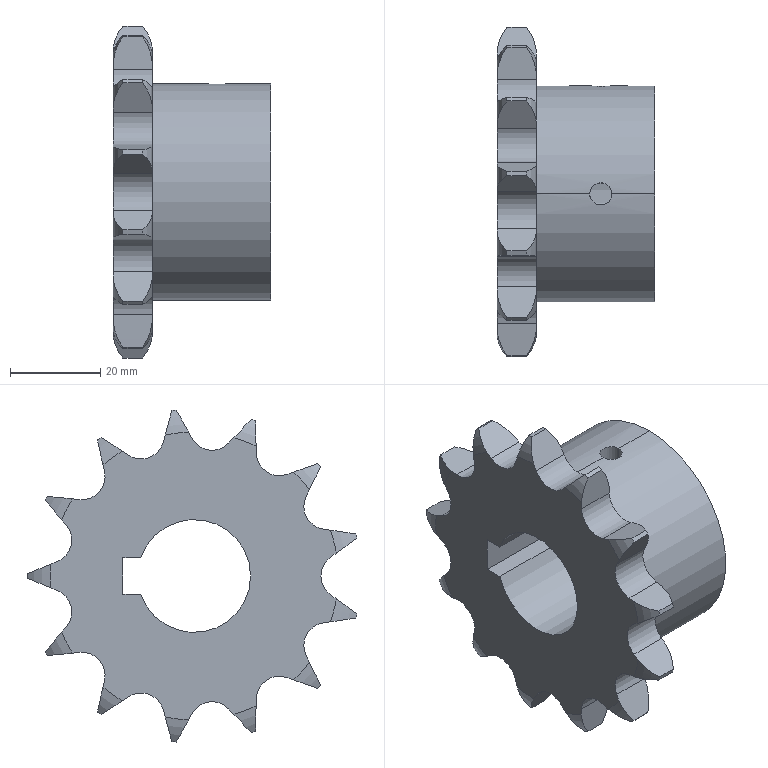Part | STEP file | DCV-000-004 | 1 solid | 93 faces | box 35 x 73.041 x 73.574 mm | volume 55395 mm3 | cylinder 35 | plane 32 | torus 26 | commonest cylinder face diameters 74 x14 10.16 x13 4.917 x4 25 x2 48 x2